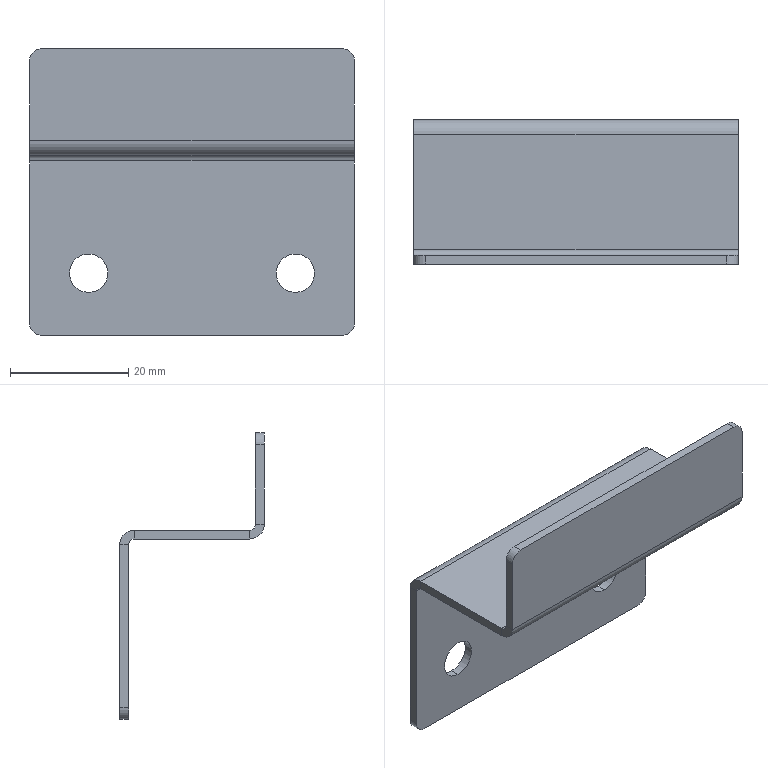Part | STEP file | 1 solid | 30 faces | box 55 x 24.5 x 48.5 mm | volume 5670 mm3 | plane 18 | cylinder 12 | commonest cylinder face diameters 4 x4 6.5 x4 2 x2 5 x2